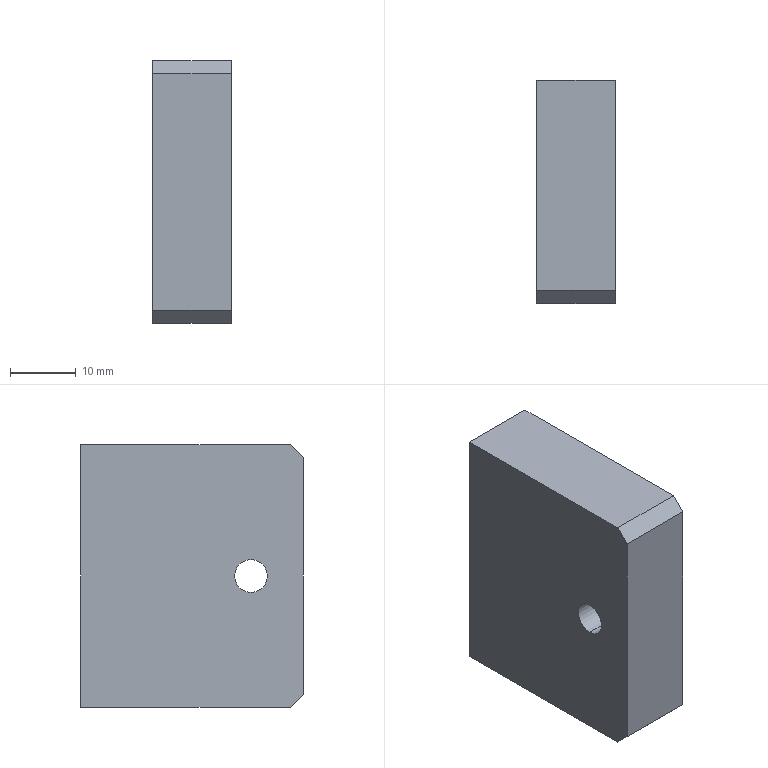Part | STEP file | PN_0037 | 1 solid | 24 faces | box 12 x 34 x 40 mm | volume 15555 mm3 | cylinder 10 | plane 10 | cone 4 | commonest cylinder face diameters 4 x4 4.2 x4 5 x2